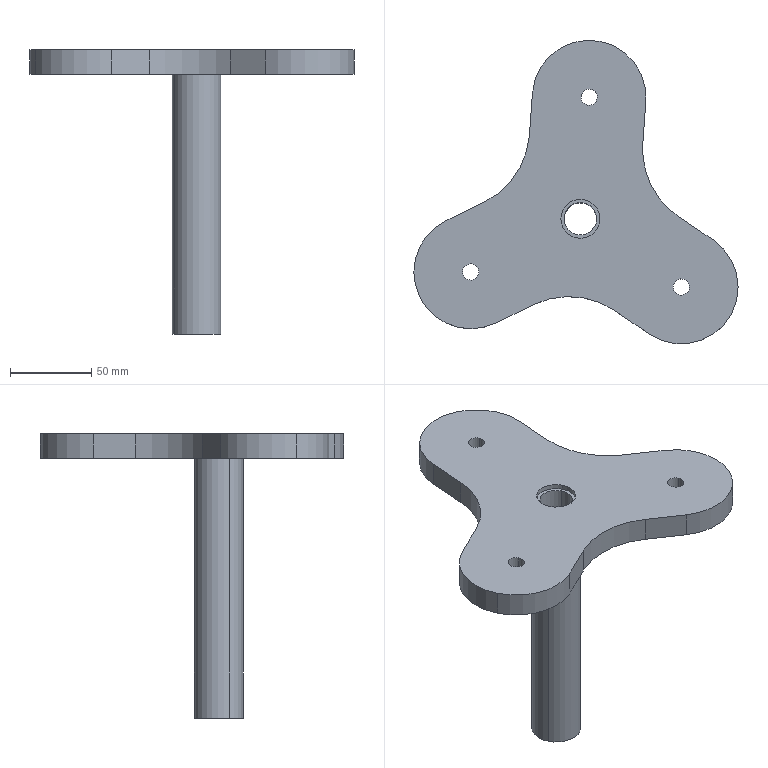Part | SolidWorks | features BaseBody 1 | 1 solid | 30 faces | box 199.568 x 186.874 x 175 mm | volume 351231 mm3 | cylinder 20 | plane 10 | commonest cylinder face diameters 10 x6 70 x4 100 x4 20 x2 24 x2 30 x2
STEP:
#1=CARTESIAN_POINT('',(-432.236,62.377,432.));
#2=VERTEX_POINT('',#1);
#3=CARTESIAN_POINT('',(-453.829,51.9,432.));
#4=VERTEX_POINT('',#3);
#5=CARTESIAN_POINT('',(-443.032,57.138,432.));
#6=DIRECTION('',(0.,0.,1.));
#7=DIRECTION('',(-0.8997,-0.4365,0.));
#8=AXIS2_PLACEMENT_3D('',#5,#6,#7);
#9=CIRCLE('',#8,12.);
#10=EDGE_CURVE('',#2,#4,#9,.T.);
#11=ORIENTED_EDGE('',*,*,#10,.F.);
#12=CARTESIAN_POINT('',(-432.236,62.377,435.));
#13=VERTEX_POINT('',#12);
#14=CARTESIAN_POINT('',(-432.236,62.377,432.));
#15=DIRECTION('',(0.,0.,1.));
#16=VECTOR('',#15,1000.);
#17=LINE('',#14,#16);
#18=EDGE_CURVE('',#2,#13,#17,.T.);
#19=ORIENTED_EDGE('',*,*,#18,.T.);
#20=CARTESIAN_POINT('',(-453.829,51.9,435.));
#21=VERTEX_POINT('',#20);
#22=CARTESIAN_POINT('',(-443.032,57.138,435.));
#23=DIRECTION('',(0.,0.,1.));
#24=DIRECTION('',(-0.8997,-0.4365,0.));
#25=AXIS2_PLACEMENT_3D('',#22,#23,#24);
#26=CIRCLE('',#25,12.);
#27=EDGE_CURVE('',#13,#21,#26,.T.);
#28=ORIENTED_EDGE('',*,*,#27,.T.);
#29=CARTESIAN_POINT('',(-453.829,51.9,432.));
#30=DIRECTION('',(0.,0.,1.));
#31=VECTOR('',#30,1000.);
#32=LINE('',#29,#31);
#33=EDGE_CURVE('',#4,#21,#32,.T.);
#34=ORIENTED_EDGE('',*,*,#33,.F.);
#35=EDGE_LOOP('',(#11,#19,#28,#34));
#36=FACE_OUTER_BOUND('',#35,.T.);
#37=CARTESIAN_POINT('',(-443.032,57.138,432.));
#38=DIRECTION('',(0.,0.,1.));
#39=DIRECTION('',(-0.8997,-0.4365,0.));
#40=AXIS2_PLACEMENT_3D('',#37,#38,#39);
#41=CYLINDRICAL_SURFACE('',#40,12.);
#42=ADVANCED_FACE('',(#36),#41,.F.);
#43=CARTESIAN_POINT('',(-429.537,63.686,260.));
#44=VERTEX_POINT('',#43);
#45=CARTESIAN_POINT('',(-456.528,50.591,260.));
#46=VERTEX_POINT('',#45);
#47=CARTESIAN_POINT('',(-443.032,57.138,260.));
#48=DIRECTION('',(0.,0.,-1.));
#49=DIRECTION('',(0.8997,0.4365,0.));
#50=AXIS2_PLACEMENT_3D('',#47,#48,#49);
#51=CIRCLE('',#50,15.);
#52=EDGE_CURVE('',#44,#46,#51,.T.);
#53=ORIENTED_EDGE('',*,*,#52,.F.);
#54=CARTESIAN_POINT('',(-429.537,63.686,420.));
#55=VERTEX_POINT('',#54);
#56=CARTESIAN_POINT('',(-429.537,63.686,330.));
#57=DIRECTION('',(0.,0.,1.));
#58=VECTOR('',#57,1000.);
#59=LINE('',#56,#58);
#60=EDGE_CURVE('',#44,#55,#59,.T.);
#61=ORIENTED_EDGE('',*,*,#60,.T.);
#62=CARTESIAN_POINT('',(-456.528,50.591,420.));
#63=VERTEX_POINT('',#62);
#64=CARTESIAN_POINT('',(-443.032,57.138,420.));
#65=DIRECTION('',(0.,0.,-1.));
#66=DIRECTION('',(0.8997,0.4365,0.));
#67=AXIS2_PLACEMENT_3D('',#64,#65,#66);
#68=CIRCLE('',#67,15.);
#69=EDGE_CURVE('',#55,#63,#68,.T.);
#70=ORIENTED_EDGE('',*,*,#69,.T.);
#71=CARTESIAN_POINT('',(-456.528,50.591,330.));
#72=DIRECTION('',(0.,0.,1.));
#73=VECTOR('',#72,1000.);
#74=LINE('',#71,#73);
#75=EDGE_CURVE('',#46,#63,#74,.T.);
#76=ORIENTED_EDGE('',*,*,#75,.F.);
#77=EDGE_LOOP('',(#53,#61,#70,#76));
#78=FACE_OUTER_BOUND('',#77,.T.);
#79=CARTESIAN_POINT('',(-443.032,57.138,330.));
#80=DIRECTION('',(0.,0.,1.));
#81=DIRECTION('',(-0.8997,-0.4365,0.));
#82=AXIS2_PLACEMENT_3D('',#79,#80,#81);
#83=CYLINDRICAL_SURFACE('',#82,15.);
#84=ADVANCED_FACE('',(#78),#83,.T.);
#85=CARTESIAN_POINT('',(-442.145,129.762,435.));
#86=VERTEX_POINT('',#85);
#87=CARTESIAN_POINT('',(-433.148,134.127,435.));
#88=VERTEX_POINT('',#87);
#89=CARTESIAN_POINT('',(-437.646,131.945,435.));
#90=DIRECTION('',(0.,0.,-1.));
#91=DIRECTION('',(0.8997,0.4365,0.));
#92=AXIS2_PLACEMENT_3D('',#89,#90,#91);
#93=CIRCLE('',#92,5.);
#94=EDGE_CURVE('',#86,#88,#93,.T.);
#95=ORIENTED_EDGE('',*,*,#94,.F.);
#96=CARTESIAN_POINT('',(-442.145,129.762,420.));
#97=VERTEX_POINT('',#96);
#98=CARTESIAN_POINT('',(-442.145,129.762,435.));
#99=DIRECTION('',(0.,0.,-1.));
#100=VECTOR('',#99,1000.);
#101=LINE('',#98,#100);
#102=EDGE_CURVE('',#86,#97,#101,.T.);
#103=ORIENTED_EDGE('',*,*,#102,.T.);
#104=CARTESIAN_POINT('',(-433.148,134.127,420.));
#105=VERTEX_POINT('',#104);
#106=CARTESIAN_POINT('',(-437.646,131.945,420.));
#107=DIRECTION('',(0.,0.,-1.));
#108=DIRECTION('',(0.8997,0.4365,0.));
#109=AXIS2_PLACEMENT_3D('',#106,#107,#108);
#110=CIRCLE('',#109,5.);
#111=EDGE_CURVE('',#97,#105,#110,.T.);
#112=ORIENTED_EDGE('',*,*,#111,.T.);
#113=CARTESIAN_POINT('',(-433.148,134.127,435.));
#114=DIRECTION('',(0.,0.,-1.));
#115=VECTOR('',#114,1000.);
#116=LINE('',#113,#115);
#117=EDGE_CURVE('',#88,#105,#116,.T.);
#118=ORIENTED_EDGE('',*,*,#117,.F.);
#119=EDGE_LOOP('',(#95,#103,#112,#118));
#120=FACE_OUTER_BOUND('',#119,.T.);
#121=CARTESIAN_POINT('',(-437.646,131.945,435.));
#122=DIRECTION('',(0.,0.,-1.));
#123=DIRECTION('',(0.8997,0.4365,0.));
#124=AXIS2_PLACEMENT_3D('',#121,#122,#123);
#125=CYLINDRICAL_SURFACE('',#124,5.);
#126=ADVANCED_FACE('',(#120),#125,.F.);
#127=CARTESIAN_POINT('',(-385.44,12.888,435.));
#128=VERTEX_POINT('',#127);
#129=CARTESIAN_POINT('',(-376.443,17.253,435.));
#130=VERTEX_POINT('',#129);
#131=CARTESIAN_POINT('',(-380.941,15.071,435.));
#132=DIRECTION('',(0.,0.,-1.));
#133=DIRECTION('',(0.8997,0.4365,0.));
#134=AXIS2_PLACEMENT_3D('',#131,#132,#133);
#135=CIRCLE('',#134,5.);
#136=EDGE_CURVE('',#128,#130,#135,.T.);
#137=ORIENTED_EDGE('',*,*,#136,.F.);
#138=CARTESIAN_POINT('',(-385.44,12.888,420.));
#139=VERTEX_POINT('',#138);
#140=CARTESIAN_POINT('',(-385.44,12.888,435.));
#141=DIRECTION('',(0.,0.,-1.));
#142=VECTOR('',#141,1000.);
#143=LINE('',#140,#142);
#144=EDGE_CURVE('',#128,#139,#143,.T.);
#145=ORIENTED_EDGE('',*,*,#144,.T.);
#146=CARTESIAN_POINT('',(-376.443,17.253,420.));
#147=VERTEX_POINT('',#146);
#148=CARTESIAN_POINT('',(-380.941,15.071,420.));
#149=DIRECTION('',(0.,0.,-1.));
#150=DIRECTION('',(0.8997,0.4365,0.));
#151=AXIS2_PLACEMENT_3D('',#148,#149,#150);
#152=CIRCLE('',#151,5.);
#153=EDGE_CURVE('',#139,#147,#152,.T.);
#154=ORIENTED_EDGE('',*,*,#153,.T.);
#155=CARTESIAN_POINT('',(-376.443,17.253,435.));
#156=DIRECTION('',(0.,0.,-1.));
#157=VECTOR('',#156,1000.);
#158=LINE('',#155,#157);
#159=EDGE_CURVE('',#130,#147,#158,.T.);
#160=ORIENTED_EDGE('',*,*,#159,.F.);
#161=EDGE_LOOP('',(#137,#145,#154,#160));
#162=FACE_OUTER_BOUND('',#161,.T.);
#163=CARTESIAN_POINT('',(-380.941,15.071,435.));
#164=DIRECTION('',(0.,0.,-1.));
#165=DIRECTION('',(0.8997,0.4365,0.));
#166=AXIS2_PLACEMENT_3D('',#163,#164,#165);
#167=CYLINDRICAL_SURFACE('',#166,5.);
#168=ADVANCED_FACE('',(#162),#167,.F.);
#169=CARTESIAN_POINT('',(-515.008,22.217,435.));
#170=VERTEX_POINT('',#169);
#171=CARTESIAN_POINT('',(-506.011,26.582,435.));
#172=VERTEX_POINT('',#171);
#173=CARTESIAN_POINT('',(-510.509,24.4,435.));
#174=DIRECTION('',(0.,0.,-1.));
#175=DIRECTION('',(0.8997,0.4365,0.));
#176=AXIS2_PLACEMENT_3D('',#173,#174,#175);
#177=CIRCLE('',#176,5.);
#178=EDGE_CURVE('',#170,#172,#177,.T.);
#179=ORIENTED_EDGE('',*,*,#178,.F.);
#180=CARTESIAN_POINT('',(-515.008,22.217,420.));
#181=VERTEX_POINT('',#180);
#182=CARTESIAN_POINT('',(-515.008,22.217,435.));
#183=DIRECTION('',(0.,0.,-1.));
#184=VECTOR('',#183,1000.);
#185=LINE('',#182,#184);
#186=EDGE_CURVE('',#170,#181,#185,.T.);
#187=ORIENTED_EDGE('',*,*,#186,.T.);
#188=CARTESIAN_POINT('',(-506.011,26.582,420.));
#189=VERTEX_POINT('',#188);
#190=CARTESIAN_POINT('',(-510.509,24.4,420.));
#191=DIRECTION('',(0.,0.,-1.));
#192=DIRECTION('',(0.8997,0.4365,0.));
#193=AXIS2_PLACEMENT_3D('',#190,#191,#192);
#194=CIRCLE('',#193,5.);
#195=EDGE_CURVE('',#181,#189,#194,.T.);
#196=ORIENTED_EDGE('',*,*,#195,.T.);
#197=CARTESIAN_POINT('',(-506.011,26.582,435.));
#198=DIRECTION('',(0.,0.,-1.));
#199=VECTOR('',#198,1000.);
#200=LINE('',#197,#199);
#201=EDGE_CURVE('',#172,#189,#200,.T.);
#202=ORIENTED_EDGE('',*,*,#201,.F.);
#203=EDGE_LOOP('',(#179,#187,#196,#202));
#204=FACE_OUTER_BOUND('',#203,.T.);
#205=CARTESIAN_POINT('',(-510.509,24.4,435.));
#206=DIRECTION('',(0.,0.,-1.));
#207=DIRECTION('',(0.8997,0.4365,0.));
#208=AXIS2_PLACEMENT_3D('',#205,#206,#207);
#209=CYLINDRICAL_SURFACE('',#208,5.);
#210=ADVANCED_FACE('',(#204),#209,.F.);
#211=CARTESIAN_POINT('',(-541.999,9.122,420.));
#212=VERTEX_POINT('',#211);
#213=CARTESIAN_POINT('',(-525.788,55.889,420.));
#214=VERTEX_POINT('',#213);
#215=CARTESIAN_POINT('',(-510.509,24.4,420.));
#216=DIRECTION('',(0.,0.,-1.));
#217=DIRECTION('',(0.8997,0.4365,0.));
#218=AXIS2_PLACEMENT_3D('',#215,#216,#217);
#219=CIRCLE('',#218,35.);
#220=EDGE_CURVE('',#212,#214,#219,.T.);
#221=ORIENTED_EDGE('',*,*,#220,.F.);
#222=CARTESIAN_POINT('',(-541.999,9.122,435.));
#223=VERTEX_POINT('',#222);
#224=CARTESIAN_POINT('',(-541.999,9.122,430.));
#225=DIRECTION('',(0.,0.,1.));
#226=VECTOR('',#225,1000.);
#227=LINE('',#224,#226);
#228=EDGE_CURVE('',#212,#223,#227,.T.);
#229=ORIENTED_EDGE('',*,*,#228,.T.);
#230=CARTESIAN_POINT('',(-525.788,55.889,435.));
#231=VERTEX_POINT('',#230);
#232=CARTESIAN_POINT('',(-510.509,24.4,435.));
#233=DIRECTION('',(0.,0.,-1.));
#234=DIRECTION('',(0.8997,0.4365,0.));
#235=AXIS2_PLACEMENT_3D('',#232,#233,#234);
#236=CIRCLE('',#235,35.);
#237=EDGE_CURVE('',#223,#231,#236,.T.);
#238=ORIENTED_EDGE('',*,*,#237,.T.);
#239=CARTESIAN_POINT('',(-525.788,55.889,430.));
#240=DIRECTION('',(0.,0.,1.));
#241=VECTOR('',#240,1000.);
#242=LINE('',#239,#241);
#243=EDGE_CURVE('',#214,#231,#242,.T.);
#244=ORIENTED_EDGE('',*,*,#243,.F.);
#245=EDGE_LOOP('',(#221,#229,#238,#244));
#246=FACE_OUTER_BOUND('',#245,.T.);
#247=CARTESIAN_POINT('',(-510.509,24.4,430.));
#248=DIRECTION('',(0.,0.,1.));
#249=DIRECTION('',(-0.8997,-0.4365,0.));
#250=AXIS2_PLACEMENT_3D('',#247,#248,#249);
#251=CYLINDRICAL_SURFACE('',#250,35.);
#252=ADVANCED_FACE('',(#246),#251,.T.);
#253=CARTESIAN_POINT('',(-399.712,78.156,420.));
#254=VERTEX_POINT('',#253);
#255=CARTESIAN_POINT('',(-382.773,58.588,420.));
#256=VERTEX_POINT('',#255);
#257=CARTESIAN_POINT('',(-354.727,99.982,420.));
#258=DIRECTION('',(0.,0.,1.));
#259=DIRECTION('',(0.8997,0.4365,0.));
#260=AXIS2_PLACEMENT_3D('',#257,#258,#259);
#261=CIRCLE('',#260,50.);
#262=EDGE_CURVE('',#254,#256,#261,.T.);
#263=ORIENTED_EDGE('',*,*,#262,.F.);
#264=CARTESIAN_POINT('',(-399.712,78.156,435.));
#265=VERTEX_POINT('',#264);
#266=CARTESIAN_POINT('',(-399.712,78.156,430.));
#267=DIRECTION('',(0.,0.,1.));
#268=VECTOR('',#267,1000.);
#269=LINE('',#266,#268);
#270=EDGE_CURVE('',#254,#265,#269,.T.);
#271=ORIENTED_EDGE('',*,*,#270,.T.);
#272=CARTESIAN_POINT('',(-382.773,58.588,435.));
#273=VERTEX_POINT('',#272);
#274=CARTESIAN_POINT('',(-354.727,99.982,435.));
#275=DIRECTION('',(0.,0.,1.));
#276=DIRECTION('',(0.8997,0.4365,0.));
#277=AXIS2_PLACEMENT_3D('',#274,#275,#276);
#278=CIRCLE('',#277,50.);
#279=EDGE_CURVE('',#265,#273,#278,.T.);
#280=ORIENTED_EDGE('',*,*,#279,.T.);
#281=CARTESIAN_POINT('',(-382.773,58.588,430.));
#282=DIRECTION('',(0.,0.,1.));
#283=VECTOR('',#282,1000.);
#284=LINE('',#281,#283);
#285=EDGE_CURVE('',#256,#273,#284,.T.);
#286=ORIENTED_EDGE('',*,*,#285,.F.);
#287=EDGE_LOOP('',(#263,#271,#280,#286));
#288=FACE_OUTER_BOUND('',#287,.T.);
#289=CARTESIAN_POINT('',(-354.727,99.982,430.));
#290=DIRECTION('',(0.,0.,1.));
#291=DIRECTION('',(-0.8997,-0.4365,0.));
#292=AXIS2_PLACEMENT_3D('',#289,#290,#291);
#293=CYLINDRICAL_SURFACE('',#292,50.);
#294=ADVANCED_FACE('',(#288),#293,.F.);
#295=CARTESIAN_POINT('',(-452.029,52.773,432.));
#296=VERTEX_POINT('',#295);
#297=CARTESIAN_POINT('',(-434.035,61.504,432.));
#298=VERTEX_POINT('',#297);
#299=CARTESIAN_POINT('',(-443.032,57.138,432.));
#300=DIRECTION('',(0.,0.,-1.));
#301=DIRECTION('',(-0.8997,-0.4365,0.));
#302=AXIS2_PLACEMENT_3D('',#299,#300,#301);
#303=CIRCLE('',#302,10.);
#304=EDGE_CURVE('',#296,#298,#303,.T.);
#305=ORIENTED_EDGE('',*,*,#304,.F.);
#306=CARTESIAN_POINT('',(-452.029,52.773,260.));
#307=VERTEX_POINT('',#306);
#308=CARTESIAN_POINT('',(-452.029,52.773,435.));
#309=DIRECTION('',(0.,0.,-1.));
#310=VECTOR('',#309,1000.);
#311=LINE('',#308,#310);
#312=EDGE_CURVE('',#296,#307,#311,.T.);
#313=ORIENTED_EDGE('',*,*,#312,.T.);
#314=CARTESIAN_POINT('',(-434.035,61.504,260.));
#315=VERTEX_POINT('',#314);
#316=CARTESIAN_POINT('',(-443.032,57.138,260.));
#317=DIRECTION('',(0.,0.,-1.));
#318=DIRECTION('',(0.8997,0.4365,0.));
#319=AXIS2_PLACEMENT_3D('',#316,#317,#318);
#320=CIRCLE('',#319,10.);
#321=EDGE_CURVE('',#307,#315,#320,.T.);
#322=ORIENTED_EDGE('',*,*,#321,.T.);
#323=CARTESIAN_POINT('',(-434.035,61.504,435.));
#324=DIRECTION('',(0.,0.,-1.));
#325=VECTOR('',#324,1000.);
#326=LINE('',#323,#325);
#327=EDGE_CURVE('',#298,#315,#326,.T.);
#328=ORIENTED_EDGE('',*,*,#327,.F.);
#329=EDGE_LOOP('',(#305,#313,#322,#328));
#330=FACE_OUTER_BOUND('',#329,.T.);
#331=CARTESIAN_POINT('',(-443.032,57.138,435.));
#332=DIRECTION('',(0.,0.,-1.));
#333=DIRECTION('',(0.8997,0.4365,0.));
#334=AXIS2_PLACEMENT_3D('',#331,#332,#333);
#335=CYLINDRICAL_SURFACE('',#334,10.);
#336=ADVANCED_FACE('',(#330),#335,.F.);
#337=ORIENTED_EDGE('',*,*,#312,.F.);
#338=CARTESIAN_POINT('',(-443.032,57.138,432.));
#339=DIRECTION('',(0.,0.,-1.));
#340=DIRECTION('',(-0.8997,-0.4365,0.));
#341=AXIS2_PLACEMENT_3D('',#338,#339,#340);
#342=CIRCLE('',#341,10.);
#343=EDGE_CURVE('',#298,#296,#342,.T.);
#344=ORIENTED_EDGE('',*,*,#343,.F.);
#345=ORIENTED_EDGE('',*,*,#327,.T.);
#346=CARTESIAN_POINT('',(-443.032,57.138,260.));
#347=DIRECTION('',(0.,0.,-1.));
#348=DIRECTION('',(0.8997,0.4365,0.));
#349=AXIS2_PLACEMENT_3D('',#346,#347,#348);
#350=CIRCLE('',#349,10.);
#351=EDGE_CURVE('',#315,#307,#350,.T.);
#352=ORIENTED_EDGE('',*,*,#351,.T.);
#353=EDGE_LOOP('',(#337,#344,#345,#352));
#354=FACE_OUTER_BOUND('',#353,.T.);
#355=CARTESIAN_POINT('',(-443.032,57.138,435.));
#356=DIRECTION('',(0.,0.,-1.));
#357=DIRECTION('',(0.8997,0.4365,0.));
#358=AXIS2_PLACEMENT_3D('',#355,#356,#357);
#359=CYLINDRICAL_SURFACE('',#358,10.);
#360=ADVANCED_FACE('',(#354),#359,.F.);
#361=CARTESIAN_POINT('',(-502.463,67.206,420.));
#362=VERTEX_POINT('',#361);
#363=CARTESIAN_POINT('',(-474.418,108.6,420.));
#364=VERTEX_POINT('',#363);
#365=CARTESIAN_POINT('',(-524.289,112.191,420.));
#366=DIRECTION('',(0.,0.,1.));
#367=DIRECTION('',(0.8997,0.4365,0.));
#368=AXIS2_PLACEMENT_3D('',#365,#366,#367);
#369=CIRCLE('',#368,50.);
#370=EDGE_CURVE('',#362,#364,#369,.T.);
#371=ORIENTED_EDGE('',*,*,#370,.T.);
#372=CARTESIAN_POINT('',(-472.556,134.458,420.));
#373=VERTEX_POINT('',#372);
#374=CARTESIAN_POINT('',(-472.556,134.458,420.));
#375=DIRECTION('',(0.07181,0.9974,0.));
#376=VECTOR('',#375,1000.);
#377=LINE('',#374,#376);
#378=EDGE_CURVE('',#364,#373,#377,.T.);
#379=ORIENTED_EDGE('',*,*,#378,.T.);
#380=CARTESIAN_POINT('',(-402.737,129.431,420.));
#381=VERTEX_POINT('',#380);
#382=CARTESIAN_POINT('',(-437.646,131.945,420.));
#383=DIRECTION('',(0.,0.,-1.));
#384=DIRECTION('',(0.8997,0.4365,0.));
#385=AXIS2_PLACEMENT_3D('',#382,#383,#384);
#386=CIRCLE('',#385,35.);
#387=EDGE_CURVE('',#373,#381,#386,.T.);
#388=ORIENTED_EDGE('',*,*,#387,.T.);
#389=CARTESIAN_POINT('',(-404.598,103.573,420.));
#390=VERTEX_POINT('',#389);
#391=CARTESIAN_POINT('',(-402.737,129.431,420.));
#392=DIRECTION('',(-0.07181,-0.9974,0.));
#393=VECTOR('',#392,1000.);
#394=LINE('',#391,#393);
#395=EDGE_CURVE('',#381,#390,#394,.T.);
#396=ORIENTED_EDGE('',*,*,#395,.T.);
#397=CARTESIAN_POINT('',(-354.727,99.982,420.));
#398=DIRECTION('',(0.,0.,1.));
#399=DIRECTION('',(0.8997,0.4365,0.));
#400=AXIS2_PLACEMENT_3D('',#397,#398,#399);
#401=CIRCLE('',#400,50.);
#402=EDGE_CURVE('',#390,#254,#401,.T.);
#403=ORIENTED_EDGE('',*,*,#402,.T.);
#404=ORIENTED_EDGE('',*,*,#262,.T.);
#405=CARTESIAN_POINT('',(-361.31,44.047,420.));
#406=VERTEX_POINT('',#405);
#407=CARTESIAN_POINT('',(-361.31,44.047,420.));
#408=DIRECTION('',(0.8279,-0.5609,0.));
#409=VECTOR('',#408,1000.);
#410=LINE('',#407,#409);
#411=EDGE_CURVE('',#256,#406,#410,.T.);
#412=ORIENTED_EDGE('',*,*,#411,.T.);
#413=CARTESIAN_POINT('',(-400.573,-13.905,420.));
#414=VERTEX_POINT('',#413);
#415=CARTESIAN_POINT('',(-380.941,15.071,420.));
#416=DIRECTION('',(0.,0.,-1.));
#417=DIRECTION('',(0.8997,0.4365,0.));
#418=AXIS2_PLACEMENT_3D('',#415,#416,#417);
#419=CIRCLE('',#418,35.);
#420=EDGE_CURVE('',#406,#414,#419,.T.);
#421=ORIENTED_EDGE('',*,*,#420,.T.);
#422=CARTESIAN_POINT('',(-422.036,0.6363,420.));
#423=VERTEX_POINT('',#422);
#424=CARTESIAN_POINT('',(-400.573,-13.905,420.));
#425=DIRECTION('',(-0.8279,0.5609,0.));
#426=VECTOR('',#425,1000.);
#427=LINE('',#424,#426);
#428=EDGE_CURVE('',#414,#423,#427,.T.);
#429=ORIENTED_EDGE('',*,*,#428,.T.);
#430=CARTESIAN_POINT('',(-471.907,4.227,420.));
#431=VERTEX_POINT('',#430);
#432=CARTESIAN_POINT('',(-450.081,-40.758,420.));
#433=DIRECTION('',(0.,0.,1.));
#434=DIRECTION('',(0.8997,0.4365,0.));
#435=AXIS2_PLACEMENT_3D('',#432,#433,#434);
#436=CIRCLE('',#435,50.);
#437=EDGE_CURVE('',#423,#431,#436,.T.);
#438=ORIENTED_EDGE('',*,*,#437,.T.);
#439=CARTESIAN_POINT('',(-495.231,-7.09,420.));
#440=VERTEX_POINT('',#439);
#441=CARTESIAN_POINT('',(-495.231,-7.09,420.));
#442=DIRECTION('',(-0.8997,-0.4365,0.));
#443=VECTOR('',#442,1000.);
#444=LINE('',#441,#443);
#445=EDGE_CURVE('',#431,#440,#444,.T.);
#446=ORIENTED_EDGE('',*,*,#445,.T.);
#447=CARTESIAN_POINT('',(-510.509,24.4,420.));
#448=DIRECTION('',(0.,0.,-1.));
#449=DIRECTION('',(0.8997,0.4365,0.));
#450=AXIS2_PLACEMENT_3D('',#447,#448,#449);
#451=CIRCLE('',#450,35.);
#452=EDGE_CURVE('',#440,#212,#451,.T.);
#453=ORIENTED_EDGE('',*,*,#452,.T.);
#454=ORIENTED_EDGE('',*,*,#220,.T.);
#455=CARTESIAN_POINT('',(-525.788,55.889,420.));
#456=DIRECTION('',(0.8997,0.4365,0.));
#457=VECTOR('',#456,1000.);
#458=LINE('',#455,#457);
#459=EDGE_CURVE('',#214,#362,#458,.T.);
#460=ORIENTED_EDGE('',*,*,#459,.T.);
#461=EDGE_LOOP('',(#371,#379,#388,#396,#403,#404,#412,#421,#429,#438,#446,#453,#454,#460));
#462=FACE_OUTER_BOUND('',#461,.T.);
#463=CARTESIAN_POINT('',(-510.509,24.4,420.));
#464=DIRECTION('',(0.,0.,-1.));
#465=DIRECTION('',(0.8997,0.4365,0.));
#466=AXIS2_PLACEMENT_3D('',#463,#464,#465);
#467=CIRCLE('',#466,5.);
#468=EDGE_CURVE('',#189,#181,#467,.T.);
#469=ORIENTED_EDGE('',*,*,#468,.F.);
#470=ORIENTED_EDGE('',*,*,#195,.F.);
#471=EDGE_LOOP('',(#469,#470));
#472=FACE_BOUND('',#471,.T.);
#473=CARTESIAN_POINT('',(-380.941,15.071,420.));
#474=DIRECTION('',(0.,0.,-1.));
#475=DIRECTION('',(0.8997,0.4365,0.));
#476=AXIS2_PLACEMENT_3D('',#473,#474,#475);
#477=CIRCLE('',#476,5.);
#478=EDGE_CURVE('',#147,#139,#477,.T.);
#479=ORIENTED_EDGE('',*,*,#478,.F.);
#480=ORIENTED_EDGE('',*,*,#153,.F.);
#481=EDGE_LOOP('',(#479,#480));
#482=FACE_BOUND('',#481,.T.);
#483=CARTESIAN_POINT('',(-437.646,131.945,420.));
#484=DIRECTION('',(0.,0.,-1.));
#485=DIRECTION('',(0.8997,0.4365,0.));
#486=AXIS2_PLACEMENT_3D('',#483,#484,#485);
#487=CIRCLE('',#486,5.);
#488=EDGE_CURVE('',#105,#97,#487,.T.);
#489=ORIENTED_EDGE('',*,*,#488,.F.);
#490=ORIENTED_EDGE('',*,*,#111,.F.);
#491=EDGE_LOOP('',(#489,#490));
#492=FACE_BOUND('',#491,.T.);
#493=CARTESIAN_POINT('',(-443.032,57.138,420.));
#494=DIRECTION('',(0.,0.,-1.));
#495=DIRECTION('',(0.8997,0.4365,0.));
#496=AXIS2_PLACEMENT_3D('',#493,#494,#495);
#497=CIRCLE('',#496,15.);
#498=EDGE_CURVE('',#63,#55,#497,.T.);
#499=ORIENTED_EDGE('',*,*,#498,.F.);
#500=ORIENTED_EDGE('',*,*,#69,.F.);
#501=EDGE_LOOP('',(#499,#500));
#502=FACE_BOUND('',#501,.T.);
#503=CARTESIAN_POINT('',(-524.289,112.191,420.));
#504=DIRECTION('',(0.,0.,-1.));
#505=DIRECTION('',(0.8997,0.4365,0.));
#506=AXIS2_PLACEMENT_3D('',#503,#504,#505);
#507=PLANE('',#506);
#508=ADVANCED_FACE('',(#462,#472,#482,#492,#502),#507,.T.);
#509=CARTESIAN_POINT('',(-502.463,67.206,435.));
#510=VERTEX_POINT('',#509);
#511=CARTESIAN_POINT('',(-474.418,108.6,435.));
#512=VERTEX_POINT('',#511);
#513=CARTESIAN_POINT('',(-524.289,112.191,435.));
#514=DIRECTION('',(0.,0.,1.));
#515=DIRECTION('',(0.8997,0.4365,0.));
#516=AXIS2_PLACEMENT_3D('',#513,#514,#515);
#517=CIRCLE('',#516,50.);
#518=EDGE_CURVE('',#510,#512,#517,.T.);
#519=ORIENTED_EDGE('',*,*,#518,.T.);
#520=CARTESIAN_POINT('',(-474.418,108.6,430.));
#521=DIRECTION('',(0.,0.,1.));
#522=VECTOR('',#521,1000.);
#523=LINE('',#520,#522);
#524=EDGE_CURVE('',#364,#512,#523,.T.);
#525=ORIENTED_EDGE('',*,*,#524,.F.);
#526=ORIENTED_EDGE('',*,*,#370,.F.);
#527=CARTESIAN_POINT('',(-502.463,67.206,430.));
#528=DIRECTION('',(0.,0.,1.));
#529=VECTOR('',#528,1000.);
#530=LINE('',#527,#529);
#531=EDGE_CURVE('',#362,#510,#530,.T.);
#532=ORIENTED_EDGE('',*,*,#531,.T.);
#533=EDGE_LOOP('',(#519,#525,#526,#532));
#534=FACE_OUTER_BOUND('',#533,.T.);
#535=CARTESIAN_POINT('',(-524.289,112.191,430.));
#536=DIRECTION('',(0.,0.,1.));
#537=DIRECTION('',(-0.8997,-0.4365,0.));
#538=AXIS2_PLACEMENT_3D('',#535,#536,#537);
#539=CYLINDRICAL_SURFACE('',#538,50.);
#540=ADVANCED_FACE('',(#534),#539,.F.);
#541=CARTESIAN_POINT('',(-472.556,134.458,435.));
#542=VERTEX_POINT('',#541);
#543=CARTESIAN_POINT('',(-472.556,134.458,435.));
#544=DIRECTION('',(0.07181,0.9974,0.));
#545=VECTOR('',#544,1000.);
#546=LINE('',#543,#545);
#547=EDGE_CURVE('',#512,#542,#546,.T.);
#548=ORIENTED_EDGE('',*,*,#547,.T.);
#549=CARTESIAN_POINT('',(-472.556,134.458,430.));
#550=DIRECTION('',(0.,0.,1.));
#551=VECTOR('',#550,1000.);
#552=LINE('',#549,#551);
#553=EDGE_CURVE('',#373,#542,#552,.T.);
#554=ORIENTED_EDGE('',*,*,#553,.F.);
#555=ORIENTED_EDGE('',*,*,#378,.F.);
#556=ORIENTED_EDGE('',*,*,#524,.T.);
#557=EDGE_LOOP('',(#548,#554,#555,#556));
#558=FACE_OUTER_BOUND('',#557,.T.);
#559=CARTESIAN_POINT('',(-472.556,134.458,430.));
#560=DIRECTION('',(0.9974,-0.07181,0.));
#561=DIRECTION('',(-0.07181,-0.9974,0.));
#562=AXIS2_PLACEMENT_3D('',#559,#560,#561);
#563=PLANE('',#562);
#564=ADVANCED_FACE('',(#558),#563,.F.);
#565=CARTESIAN_POINT('',(-402.737,129.431,435.));
#566=VERTEX_POINT('',#565);
#567=CARTESIAN_POINT('',(-437.646,131.945,435.));
#568=DIRECTION('',(0.,0.,-1.));
#569=DIRECTION('',(0.8997,0.4365,0.));
#570=AXIS2_PLACEMENT_3D('',#567,#568,#569);
#571=CIRCLE('',#570,35.);
#572=EDGE_CURVE('',#542,#566,#571,.T.);
#573=ORIENTED_EDGE('',*,*,#572,.T.);
#574=CARTESIAN_POINT('',(-402.737,129.431,430.));
#575=DIRECTION('',(0.,0.,1.));
#576=VECTOR('',#575,1000.);
#577=LINE('',#574,#576);
#578=EDGE_CURVE('',#381,#566,#577,.T.);
#579=ORIENTED_EDGE('',*,*,#578,.F.);
#580=ORIENTED_EDGE('',*,*,#387,.F.);
#581=ORIENTED_EDGE('',*,*,#553,.T.);
#582=EDGE_LOOP('',(#573,#579,#580,#581));
#583=FACE_OUTER_BOUND('',#582,.T.);
#584=CARTESIAN_POINT('',(-437.646,131.945,430.));
#585=DIRECTION('',(0.,0.,1.));
#586=DIRECTION('',(-0.8997,-0.4365,0.));
#587=AXIS2_PLACEMENT_3D('',#584,#585,#586);
#588=CYLINDRICAL_SURFACE('',#587,35.);
#589=ADVANCED_FACE('',(#583),#588,.T.);
#590=CARTESIAN_POINT('',(-404.598,103.573,435.));
#591=VERTEX_POINT('',#590);
#592=CARTESIAN_POINT('',(-402.737,129.431,435.));
#593=DIRECTION('',(-0.07181,-0.9974,0.));
#594=VECTOR('',#593,1000.);
#595=LINE('',#592,#594);
#596=EDGE_CURVE('',#566,#591,#595,.T.);
#597=ORIENTED_EDGE('',*,*,#596,.T.);
#598=CARTESIAN_POINT('',(-404.598,103.573,430.));
#599=DIRECTION('',(0.,0.,1.));
#600=VECTOR('',#599,1000.);
#601=LINE('',#598,#600);
#602=EDGE_CURVE('',#390,#591,#601,.T.);
#603=ORIENTED_EDGE('',*,*,#602,.F.);
#604=ORIENTED_EDGE('',*,*,#395,.F.);
#605=ORIENTED_EDGE('',*,*,#578,.T.);
#606=EDGE_LOOP('',(#597,#603,#604,#605));
#607=FACE_OUTER_BOUND('',#606,.T.);
#608=CARTESIAN_POINT('',(-402.737,129.431,430.));
#609=DIRECTION('',(-0.9974,0.07181,0.));
#610=DIRECTION('',(0.07181,0.9974,0.));
#611=AXIS2_PLACEMENT_3D('',#608,#609,#610);
#612=PLANE('',#611);
#613=ADVANCED_FACE('',(#607),#612,.F.);
#614=ORIENTED_EDGE('',*,*,#270,.F.);
#615=ORIENTED_EDGE('',*,*,#402,.F.);
#616=ORIENTED_EDGE('',*,*,#602,.T.);
#617=CARTESIAN_POINT('',(-354.727,99.982,435.));
#618=DIRECTION('',(0.,0.,1.));
#619=DIRECTION('',(0.8997,0.4365,0.));
#620=AXIS2_PLACEMENT_3D('',#617,#618,#619);
#621=CIRCLE('',#620,50.);
#622=EDGE_CURVE('',#591,#265,#621,.T.);
#623=ORIENTED_EDGE('',*,*,#622,.T.);
#624=EDGE_LOOP('',(#614,#615,#616,#623));
#625=FACE_OUTER_BOUND('',#624,.T.);
#626=CARTESIAN_POINT('',(-354.727,99.982,430.));
#627=DIRECTION('',(0.,0.,1.));
#628=DIRECTION('',(-0.8997,-0.4365,0.));
#629=AXIS2_PLACEMENT_3D('',#626,#627,#628);
#630=CYLINDRICAL_SURFACE('',#629,50.);
#631=ADVANCED_FACE('',(#625),#630,.F.);
#632=CARTESIAN_POINT('',(-361.31,44.047,435.));
#633=VERTEX_POINT('',#632);
#634=CARTESIAN_POINT('',(-361.31,44.047,435.));
#635=DIRECTION('',(0.8279,-0.5609,0.));
#636=VECTOR('',#635,1000.);
#637=LINE('',#634,#636);
#638=EDGE_CURVE('',#273,#633,#637,.T.);
#639=ORIENTED_EDGE('',*,*,#638,.T.);
#640=CARTESIAN_POINT('',(-361.31,44.047,430.));
#641=DIRECTION('',(0.,0.,1.));
#642=VECTOR('',#641,1000.);
#643=LINE('',#640,#642);
#644=EDGE_CURVE('',#406,#633,#643,.T.);
#645=ORIENTED_EDGE('',*,*,#644,.F.);
#646=ORIENTED_EDGE('',*,*,#411,.F.);
#647=ORIENTED_EDGE('',*,*,#285,.T.);
#648=EDGE_LOOP('',(#639,#645,#646,#647));
#649=FACE_OUTER_BOUND('',#648,.T.);
#650=CARTESIAN_POINT('',(-361.31,44.047,430.));
#651=DIRECTION('',(-0.5609,-0.8279,0.));
#652=DIRECTION('',(-0.8279,0.5609,0.));
#653=AXIS2_PLACEMENT_3D('',#650,#651,#652);
#654=PLANE('',#653);
#655=ADVANCED_FACE('',(#649),#654,.F.);
#656=CARTESIAN_POINT('',(-400.573,-13.905,435.));
#657=VERTEX_POINT('',#656);
#658=CARTESIAN_POINT('',(-380.941,15.071,435.));
#659=DIRECTION('',(0.,0.,-1.));
#660=DIRECTION('',(0.8997,0.4365,0.));
#661=AXIS2_PLACEMENT_3D('',#658,#659,#660);
#662=CIRCLE('',#661,35.);
#663=EDGE_CURVE('',#633,#657,#662,.T.);
#664=ORIENTED_EDGE('',*,*,#663,.T.);
#665=CARTESIAN_POINT('',(-400.573,-13.905,430.));
#666=DIRECTION('',(0.,0.,1.));
#667=VECTOR('',#666,1000.);
#668=LINE('',#665,#667);
#669=EDGE_CURVE('',#414,#657,#668,.T.);
#670=ORIENTED_EDGE('',*,*,#669,.F.);
#671=ORIENTED_EDGE('',*,*,#420,.F.);
#672=ORIENTED_EDGE('',*,*,#644,.T.);
#673=EDGE_LOOP('',(#664,#670,#671,#672));
#674=FACE_OUTER_BOUND('',#673,.T.);
#675=CARTESIAN_POINT('',(-380.941,15.071,430.));
#676=DIRECTION('',(0.,0.,1.));
#677=DIRECTION('',(-0.8997,-0.4365,0.));
#678=AXIS2_PLACEMENT_3D('',#675,#676,#677);
#679=CYLINDRICAL_SURFACE('',#678,35.);
#680=ADVANCED_FACE('',(#674),#679,.T.);
#681=CARTESIAN_POINT('',(-422.036,0.6363,435.));
#682=VERTEX_POINT('',#681);
#683=CARTESIAN_POINT('',(-400.573,-13.905,435.));
#684=DIRECTION('',(-0.8279,0.5609,0.));
#685=VECTOR('',#684,1000.);
#686=LINE('',#683,#685);
#687=EDGE_CURVE('',#657,#682,#686,.T.);
#688=ORIENTED_EDGE('',*,*,#687,.T.);
#689=CARTESIAN_POINT('',(-422.036,0.6363,430.));
#690=DIRECTION('',(0.,0.,1.));
#691=VECTOR('',#690,1000.);
#692=LINE('',#689,#691);
#693=EDGE_CURVE('',#423,#682,#692,.T.);
#694=ORIENTED_EDGE('',*,*,#693,.F.);
#695=ORIENTED_EDGE('',*,*,#428,.F.);
#696=ORIENTED_EDGE('',*,*,#669,.T.);
#697=EDGE_LOOP('',(#688,#694,#695,#696));
#698=FACE_OUTER_BOUND('',#697,.T.);
#699=CARTESIAN_POINT('',(-400.573,-13.905,430.));
#700=DIRECTION('',(0.5609,0.8279,0.));
#701=DIRECTION('',(0.8279,-0.5609,0.));
#702=AXIS2_PLACEMENT_3D('',#699,#700,#701);
#703=PLANE('',#702);
#704=ADVANCED_FACE('',(#698),#703,.F.);
#705=CARTESIAN_POINT('',(-471.907,4.227,435.));
#706=VERTEX_POINT('',#705);
#707=CARTESIAN_POINT('',(-450.081,-40.758,435.));
#708=DIRECTION('',(0.,0.,1.));
#709=DIRECTION('',(0.8997,0.4365,0.));
#710=AXIS2_PLACEMENT_3D('',#707,#708,#709);
#711=CIRCLE('',#710,50.);
#712=EDGE_CURVE('',#682,#706,#711,.T.);
#713=ORIENTED_EDGE('',*,*,#712,.T.);
#714=CARTESIAN_POINT('',(-471.907,4.227,430.));
#715=DIRECTION('',(0.,0.,1.));
#716=VECTOR('',#715,1000.);
#717=LINE('',#714,#716);
#718=EDGE_CURVE('',#431,#706,#717,.T.);
#719=ORIENTED_EDGE('',*,*,#718,.F.);
#720=ORIENTED_EDGE('',*,*,#437,.F.);
#721=ORIENTED_EDGE('',*,*,#693,.T.);
#722=EDGE_LOOP('',(#713,#719,#720,#721));
#723=FACE_OUTER_BOUND('',#722,.T.);
#724=CARTESIAN_POINT('',(-450.081,-40.758,430.));
#725=DIRECTION('',(0.,0.,1.));
#726=DIRECTION('',(-0.8997,-0.4365,0.));
#727=AXIS2_PLACEMENT_3D('',#724,#725,#726);
#728=CYLINDRICAL_SURFACE('',#727,50.);
#729=ADVANCED_FACE('',(#723),#728,.F.);
#730=CARTESIAN_POINT('',(-495.231,-7.09,435.));
#731=VERTEX_POINT('',#730);
#732=CARTESIAN_POINT('',(-495.231,-7.09,435.));
#733=DIRECTION('',(-0.8997,-0.4365,0.));
#734=VECTOR('',#733,1000.);
#735=LINE('',#732,#734);
#736=EDGE_CURVE('',#706,#731,#735,.T.);
#737=ORIENTED_EDGE('',*,*,#736,.T.);
#738=CARTESIAN_POINT('',(-495.231,-7.09,430.));
#739=DIRECTION('',(0.,0.,1.));
#740=VECTOR('',#739,1000.);
#741=LINE('',#738,#740);
#742=EDGE_CURVE('',#440,#731,#741,.T.);
#743=ORIENTED_EDGE('',*,*,#742,.F.);
#744=ORIENTED_EDGE('',*,*,#445,.F.);
#745=ORIENTED_EDGE('',*,*,#718,.T.);
#746=EDGE_LOOP('',(#737,#743,#744,#745));
#747=FACE_OUTER_BOUND('',#746,.T.);
#748=CARTESIAN_POINT('',(-495.231,-7.09,430.));
#749=DIRECTION('',(-0.4365,0.8997,0.));
#750=DIRECTION('',(0.8997,0.4365,0.));
#751=AXIS2_PLACEMENT_3D('',#748,#749,#750);
#752=PLANE('',#751);
#753=ADVANCED_FACE('',(#747),#752,.F.);
#754=ORIENTED_EDGE('',*,*,#228,.F.);
#755=ORIENTED_EDGE('',*,*,#452,.F.);
#756=ORIENTED_EDGE('',*,*,#742,.T.);
#757=CARTESIAN_POINT('',(-510.509,24.4,435.));
#758=DIRECTION('',(0.,0.,-1.));
#759=DIRECTION('',(0.8997,0.4365,0.));
#760=AXIS2_PLACEMENT_3D('',#757,#758,#759);
#761=CIRCLE('',#760,35.);
#762=EDGE_CURVE('',#731,#223,#761,.T.);
#763=ORIENTED_EDGE('',*,*,#762,.T.);
#764=EDGE_LOOP('',(#754,#755,#756,#763));
#765=FACE_OUTER_BOUND('',#764,.T.);
#766=CARTESIAN_POINT('',(-510.509,24.4,430.));
#767=DIRECTION('',(0.,0.,1.));
#768=DIRECTION('',(-0.8997,-0.4365,0.));
#769=AXIS2_PLACEMENT_3D('',#766,#767,#768);
#770=CYLINDRICAL_SURFACE('',#769,35.);
#771=ADVANCED_FACE('',(#765),#770,.T.);
#772=CARTESIAN_POINT('',(-525.788,55.889,435.));
#773=DIRECTION('',(0.8997,0.4365,0.));
#774=VECTOR('',#773,1000.);
#775=LINE('',#772,#774);
#776=EDGE_CURVE('',#231,#510,#775,.T.);
#777=ORIENTED_EDGE('',*,*,#776,.T.);
#778=ORIENTED_EDGE('',*,*,#531,.F.);
#779=ORIENTED_EDGE('',*,*,#459,.F.);
#780=ORIENTED_EDGE('',*,*,#243,.T.);
#781=EDGE_LOOP('',(#777,#778,#779,#780));
#782=FACE_OUTER_BOUND('',#781,.T.);
#783=CARTESIAN_POINT('',(-525.788,55.889,430.));
#784=DIRECTION('',(0.4365,-0.8997,0.));
#785=DIRECTION('',(-0.8997,-0.4365,0.));
#786=AXIS2_PLACEMENT_3D('',#783,#784,#785);
#787=PLANE('',#786);
#788=ADVANCED_FACE('',(#782),#787,.F.);
#789=CARTESIAN_POINT('',(-443.032,57.138,435.));
#790=DIRECTION('',(0.,0.,1.));
#791=DIRECTION('',(-0.8997,-0.4365,0.));
#792=AXIS2_PLACEMENT_3D('',#789,#790,#791);
#793=CIRCLE('',#792,12.);
#794=EDGE_CURVE('',#21,#13,#793,.T.);
#795=ORIENTED_EDGE('',*,*,#794,.F.);
#796=ORIENTED_EDGE('',*,*,#27,.F.);
#797=EDGE_LOOP('',(#795,#796));
#798=FACE_BOUND('',#797,.T.);
#799=CARTESIAN_POINT('',(-437.646,131.945,435.));
#800=DIRECTION('',(0.,0.,-1.));
#801=DIRECTION('',(0.8997,0.4365,0.));
#802=AXIS2_PLACEMENT_3D('',#799,#800,#801);
#803=CIRCLE('',#802,5.);
#804=EDGE_CURVE('',#88,#86,#803,.T.);
#805=ORIENTED_EDGE('',*,*,#804,.T.);
#806=ORIENTED_EDGE('',*,*,#94,.T.);
#807=EDGE_LOOP('',(#805,#806));
#808=FACE_BOUND('',#807,.T.);
#809=CARTESIAN_POINT('',(-380.941,15.071,435.));
#810=DIRECTION('',(0.,0.,-1.));
#811=DIRECTION('',(0.8997,0.4365,0.));
#812=AXIS2_PLACEMENT_3D('',#809,#810,#811);
#813=CIRCLE('',#812,5.);
#814=EDGE_CURVE('',#130,#128,#813,.T.);
#815=ORIENTED_EDGE('',*,*,#814,.T.);
#816=ORIENTED_EDGE('',*,*,#136,.T.);
#817=EDGE_LOOP('',(#815,#816));
#818=FACE_BOUND('',#817,.T.);
#819=CARTESIAN_POINT('',(-510.509,24.4,435.));
#820=DIRECTION('',(0.,0.,-1.));
#821=DIRECTION('',(0.8997,0.4365,0.));
#822=AXIS2_PLACEMENT_3D('',#819,#820,#821);
#823=CIRCLE('',#822,5.);
#824=EDGE_CURVE('',#172,#170,#823,.T.);
#825=ORIENTED_EDGE('',*,*,#824,.T.);
#826=ORIENTED_EDGE('',*,*,#178,.T.);
#827=EDGE_LOOP('',(#825,#826));
#828=FACE_BOUND('',#827,.T.);
#829=ORIENTED_EDGE('',*,*,#518,.F.);
#830=ORIENTED_EDGE('',*,*,#776,.F.);
#831=ORIENTED_EDGE('',*,*,#237,.F.);
#832=ORIENTED_EDGE('',*,*,#762,.F.);
#833=ORIENTED_EDGE('',*,*,#736,.F.);
#834=ORIENTED_EDGE('',*,*,#712,.F.);
#835=ORIENTED_EDGE('',*,*,#687,.F.);
#836=ORIENTED_EDGE('',*,*,#663,.F.);
#837=ORIENTED_EDGE('',*,*,#638,.F.);
#838=ORIENTED_EDGE('',*,*,#279,.F.);
#839=ORIENTED_EDGE('',*,*,#622,.F.);
#840=ORIENTED_EDGE('',*,*,#596,.F.);
#841=ORIENTED_EDGE('',*,*,#572,.F.);
#842=ORIENTED_EDGE('',*,*,#547,.F.);
#843=EDGE_LOOP('',(#829,#830,#831,#832,#833,#834,#835,#836,#837,#838,#839,#840,#841,#842));
#844=FACE_OUTER_BOUND('',#843,.T.);
#845=CARTESIAN_POINT('',(-524.289,112.191,435.));
#846=DIRECTION('',(0.,0.,-1.));
#847=DIRECTION('',(0.8997,0.4365,0.));
#848=AXIS2_PLACEMENT_3D('',#845,#846,#847);
#849=PLANE('',#848);
#850=ADVANCED_FACE('',(#798,#808,#818,#828,#844),#849,.F.);
#851=ORIENTED_EDGE('',*,*,#186,.F.);
#852=ORIENTED_EDGE('',*,*,#824,.F.);
#853=ORIENTED_EDGE('',*,*,#201,.T.);
#854=ORIENTED_EDGE('',*,*,#468,.T.);
#855=EDGE_LOOP('',(#851,#852,#853,#854));
#856=FACE_OUTER_BOUND('',#855,.T.);
#857=CARTESIAN_POINT('',(-510.509,24.4,435.));
#858=DIRECTION('',(0.,0.,-1.));
#859=DIRECTION('',(0.8997,0.4365,0.));
#860=AXIS2_PLACEMENT_3D('',#857,#858,#859);
#861=CYLINDRICAL_SURFACE('',#860,5.);
#862=ADVANCED_FACE('',(#856),#861,.F.);
#863=ORIENTED_EDGE('',*,*,#144,.F.);
#864=ORIENTED_EDGE('',*,*,#814,.F.);
#865=ORIENTED_EDGE('',*,*,#159,.T.);
#866=ORIENTED_EDGE('',*,*,#478,.T.);
#867=EDGE_LOOP('',(#863,#864,#865,#866));
#868=FACE_OUTER_BOUND('',#867,.T.);
#869=CARTESIAN_POINT('',(-380.941,15.071,435.));
#870=DIRECTION('',(0.,0.,-1.));
#871=DIRECTION('',(0.8997,0.4365,0.));
#872=AXIS2_PLACEMENT_3D('',#869,#870,#871);
#873=CYLINDRICAL_SURFACE('',#872,5.);
#874=ADVANCED_FACE('',(#868),#873,.F.);
#875=ORIENTED_EDGE('',*,*,#102,.F.);
#876=ORIENTED_EDGE('',*,*,#804,.F.);
#877=ORIENTED_EDGE('',*,*,#117,.T.);
#878=ORIENTED_EDGE('',*,*,#488,.T.);
#879=EDGE_LOOP('',(#875,#876,#877,#878));
#880=FACE_OUTER_BOUND('',#879,.T.);
#881=CARTESIAN_POINT('',(-437.646,131.945,435.));
#882=DIRECTION('',(0.,0.,-1.));
#883=DIRECTION('',(0.8997,0.4365,0.));
#884=AXIS2_PLACEMENT_3D('',#881,#882,#883);
#885=CYLINDRICAL_SURFACE('',#884,5.);
#886=ADVANCED_FACE('',(#880),#885,.F.);
#887=CARTESIAN_POINT('',(-443.032,57.138,260.));
#888=DIRECTION('',(0.,0.,-1.));
#889=DIRECTION('',(0.8997,0.4365,0.));
#890=AXIS2_PLACEMENT_3D('',#887,#888,#889);
#891=CIRCLE('',#890,15.);
#892=EDGE_CURVE('',#46,#44,#891,.T.);
#893=ORIENTED_EDGE('',*,*,#892,.T.);
#894=ORIENTED_EDGE('',*,*,#52,.T.);
#895=EDGE_LOOP('',(#893,#894));
#896=FACE_OUTER_BOUND('',#895,.T.);
#897=ORIENTED_EDGE('',*,*,#351,.F.);
#898=ORIENTED_EDGE('',*,*,#321,.F.);
#899=EDGE_LOOP('',(#897,#898));
#900=FACE_BOUND('',#899,.T.);
#901=CARTESIAN_POINT('',(-443.032,57.138,260.));
#902=DIRECTION('',(0.,0.,-1.));
#903=DIRECTION('',(0.8997,0.4365,0.));
#904=AXIS2_PLACEMENT_3D('',#901,#902,#903);
#905=PLANE('',#904);
#906=ADVANCED_FACE('',(#896,#900),#905,.T.);
#907=ORIENTED_EDGE('',*,*,#60,.F.);
#908=ORIENTED_EDGE('',*,*,#892,.F.);
#909=ORIENTED_EDGE('',*,*,#75,.T.);
#910=ORIENTED_EDGE('',*,*,#498,.T.);
#911=EDGE_LOOP('',(#907,#908,#909,#910));
#912=FACE_OUTER_BOUND('',#911,.T.);
#913=CARTESIAN_POINT('',(-443.032,57.138,330.));
#914=DIRECTION('',(0.,0.,1.));
#915=DIRECTION('',(-0.8997,-0.4365,0.));
#916=AXIS2_PLACEMENT_3D('',#913,#914,#915);
#917=CYLINDRICAL_SURFACE('',#916,15.);
#918=ADVANCED_FACE('',(#912),#917,.T.);
#919=CARTESIAN_POINT('',(-443.032,57.138,432.));
#920=DIRECTION('',(0.,0.,1.));
#921=DIRECTION('',(-0.8997,-0.4365,0.));
#922=AXIS2_PLACEMENT_3D('',#919,#920,#921);
#923=CIRCLE('',#922,12.);
#924=EDGE_CURVE('',#4,#2,#923,.T.);
#925=ORIENTED_EDGE('',*,*,#924,.T.);
#926=ORIENTED_EDGE('',*,*,#10,.T.);
#927=EDGE_LOOP('',(#925,#926));
#928=FACE_OUTER_BOUND('',#927,.T.);
#929=ORIENTED_EDGE('',*,*,#343,.T.);
#930=ORIENTED_EDGE('',*,*,#304,.T.);
#931=EDGE_LOOP('',(#929,#930));
#932=FACE_BOUND('',#931,.T.);
#933=CARTESIAN_POINT('',(-443.032,57.138,432.));
#934=DIRECTION('',(0.,0.,1.));
#935=DIRECTION('',(-0.8997,-0.4365,0.));
#936=AXIS2_PLACEMENT_3D('',#933,#934,#935);
#937=PLANE('',#936);
#938=ADVANCED_FACE('',(#928,#932),#937,.T.);
#939=ORIENTED_EDGE('',*,*,#18,.F.);
#940=ORIENTED_EDGE('',*,*,#924,.F.);
#941=ORIENTED_EDGE('',*,*,#33,.T.);
#942=ORIENTED_EDGE('',*,*,#794,.T.);
#943=EDGE_LOOP('',(#939,#940,#941,#942));
#944=FACE_OUTER_BOUND('',#943,.T.);
#945=CARTESIAN_POINT('',(-443.032,57.138,432.));
#946=DIRECTION('',(0.,0.,1.));
#947=DIRECTION('',(-0.8997,-0.4365,0.));
#948=AXIS2_PLACEMENT_3D('',#945,#946,#947);
#949=CYLINDRICAL_SURFACE('',#948,12.);
#950=ADVANCED_FACE('',(#944),#949,.F.);
#951=CLOSED_SHELL('',(#42,#84,#126,#168,#210,#252,#294,#336,#360,#508,#540,#564,#589,#613,#631,#655,#680,#704,#729,#753,#771,#788,#850,#862,#874,#886,#906,#918,#938,#950));
#952=MANIFOLD_SOLID_BREP('',#951);
#953=CARTESIAN_POINT('',(0.,0.,0.));
#954=DIRECTION('',(0.,0.,1.));
#955=DIRECTION('',(1.,0.,0.));
#956=AXIS2_PLACEMENT_3D('',#953,#954,#955);
#957=(LENGTH_UNIT()NAMED_UNIT(*)SI_UNIT(.MILLI.,.METRE.));
#958=UNCERTAINTY_MEASURE_WITH_UNIT(LENGTH_MEASURE(0.00001),#957,'','');
#959=(NAMED_UNIT(*)PLANE_ANGLE_UNIT()SI_UNIT($,.RADIAN.));
#960=(NAMED_UNIT(*)SI_UNIT($,.STERADIAN.)SOLID_ANGLE_UNIT());
#961=(GEOMETRIC_REPRESENTATION_CONTEXT(3)GLOBAL_UNCERTAINTY_ASSIGNED_CONTEXT((#958))GLOBAL_UNIT_ASSIGNED_CONTEXT((#957,#959,#960))REPRESENTATION_CONTEXT('',''));
#962=ADVANCED_BREP_SHAPE_REPRESENTATION('',(#952,#956),#961);